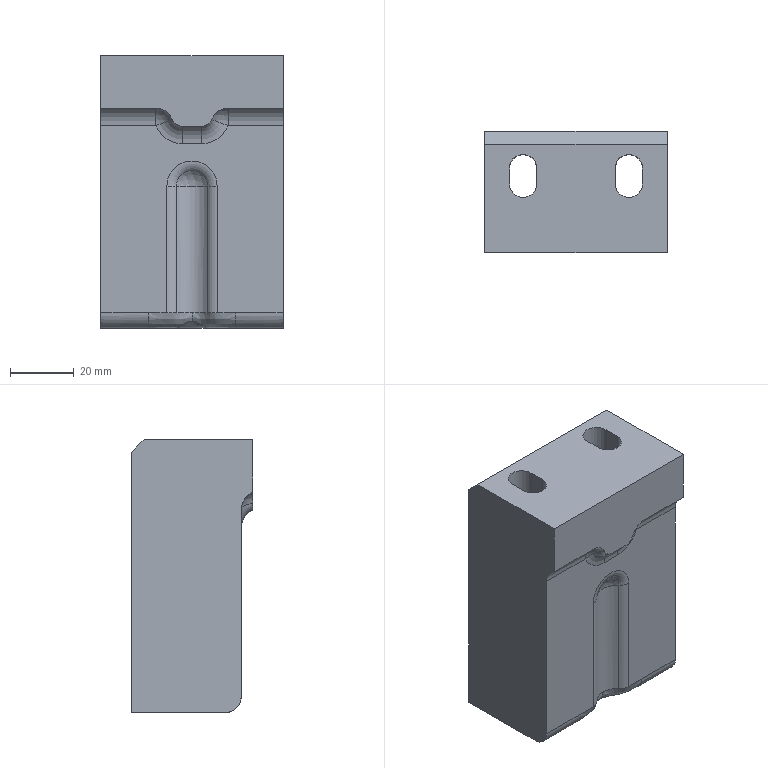Part | STEP file | 1_id50_x_t | 1 solid | 55 faces | box 57.15 x 38 x 85.5 mm | volume 143205 mm3 | plane 24 | cylinder 18 | torus 6 | sphere 3 | spline 2 | other 2 | commonest cylinder face diameters 8.5 x4 14 x4 12 x3 2 x2 8 x2 10 x2